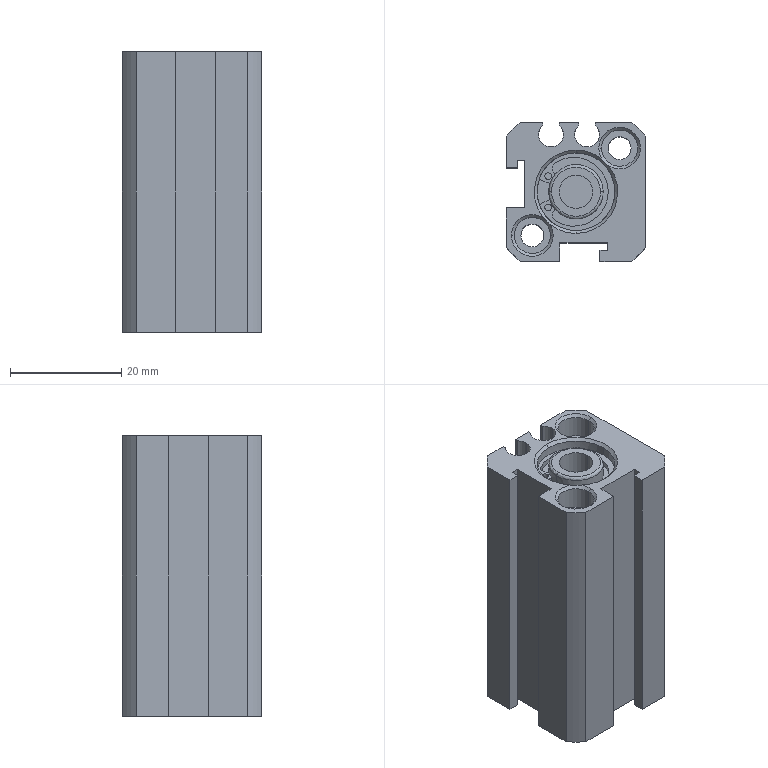Part | SolidWorks | features BaseBody 1 | 1 solid | 149 faces | box 25 x 25 x 50.5 mm | volume 19687 mm3 | cylinder 75 | plane 54 | cone 16 | spline 4 | commonest cylinder face diameters 2.4 x14 4.134 x12 1.2 x8 6.5 x8 4.5 x6 1.5 x4